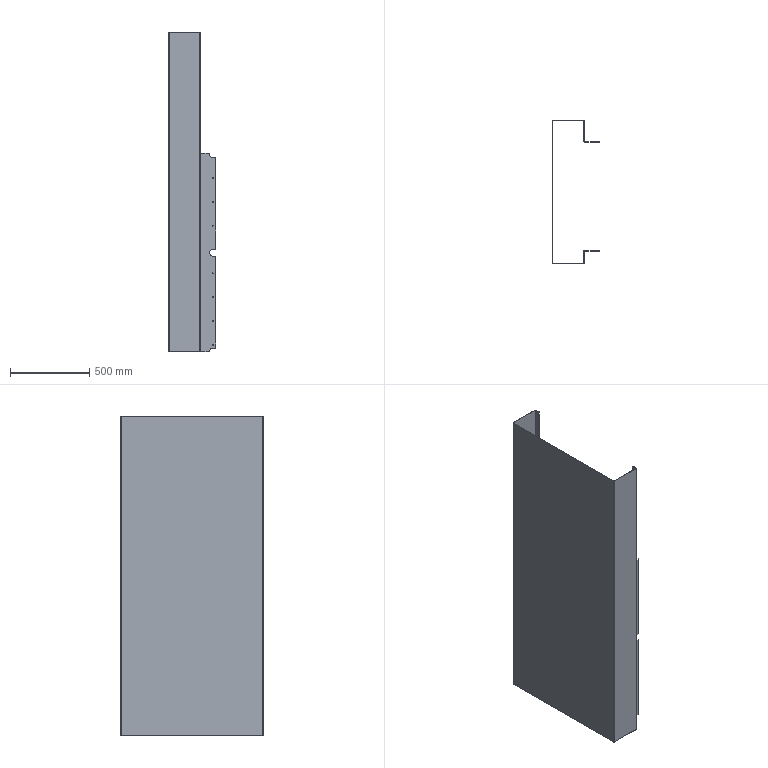Part | STEP file | C1 | 1 solid | 69 faces | box 298.717 x 900 x 2010 mm | volume 4692484 mm3 | plane 37 | cylinder 32 | commonest cylinder face diameters 7 x18 45 x6 4 x4 6 x2 10 x2